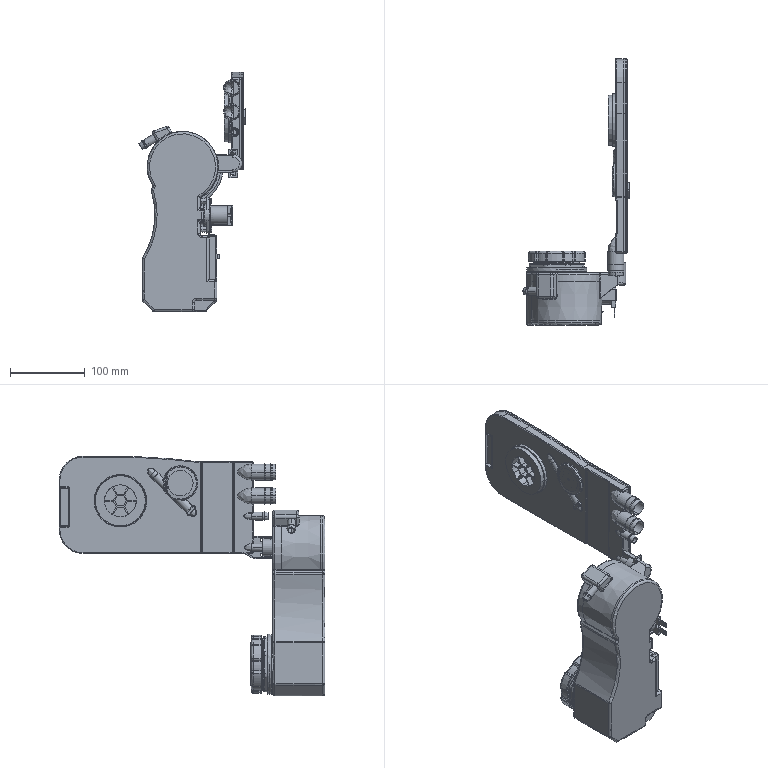Part | STEP file | ZXW722-L-76_SP | 55 solids | 4599 faces | volume 2020809 mm3 | plane 1915 | cylinder 1332 | spline 492 | torus 320 | cone 298 | sphere 129 | other 113 | commonest cylinder face diameters 2 x313 0.389 x96 0.39 x96 1 x91 6 x74 3 x48